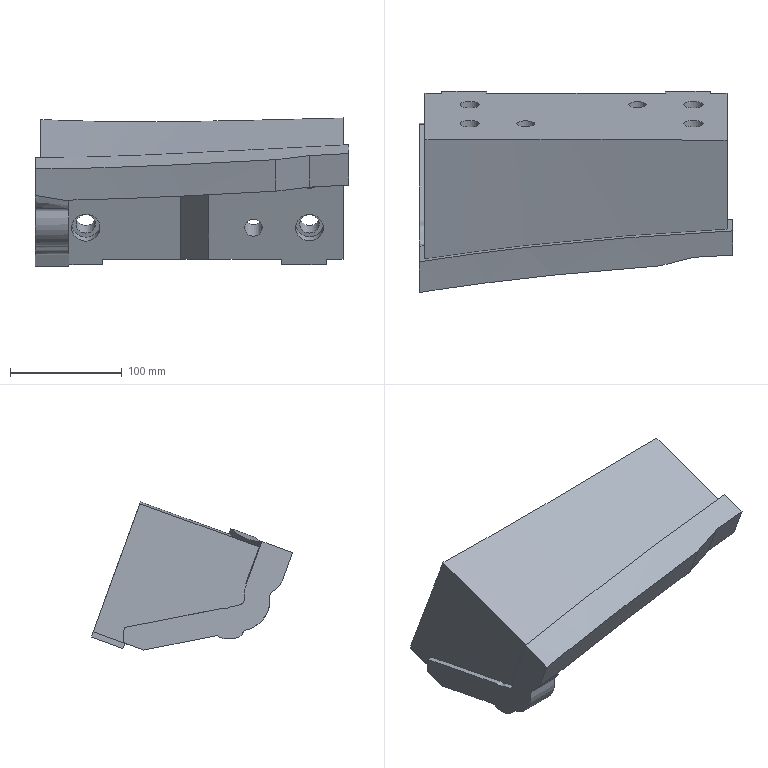Part | NX | features solid 2 | 1 solid | 46 faces | box 280 x 179.845 x 132.345 mm | volume 1948540 mm3 | plane 24 | spline 12 | cylinder 10 | commonest cylinder face diameters 17.5 x4 25 x3 16 x2 25.5 x1